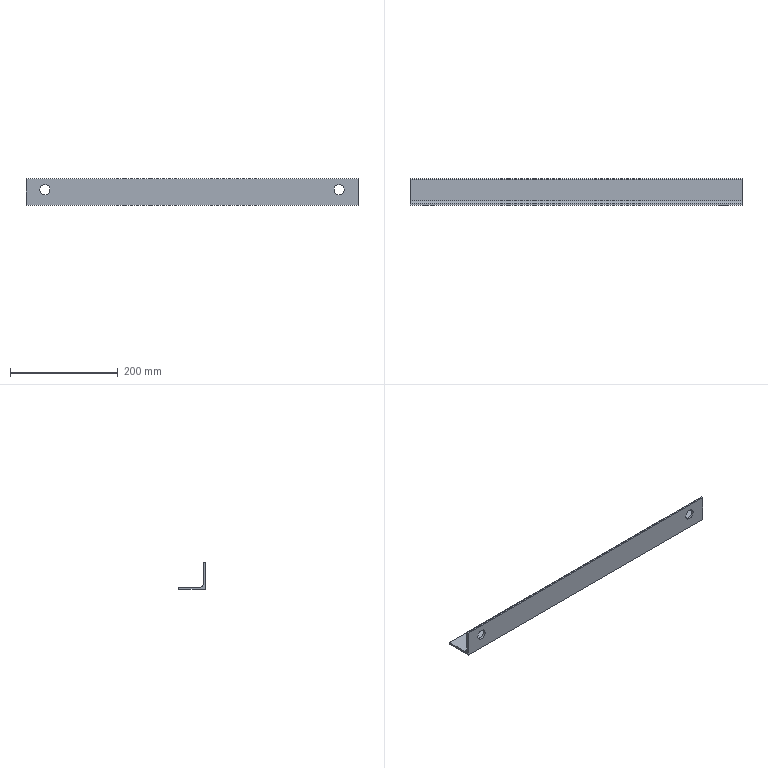Part | STEP file | Electrical cabinet angle steel 1_Default<As Machined> | 1 solid | 15 faces | box 617.5 x 50 x 50 mm | volume 238392 mm3 | plane 8 | cylinder 7 | commonest cylinder face diameters 19 x4 2.66 x2 11 x1
STEP:
#1=CARTESIAN_POINT('',(0.,0.,0.));
#2=DIRECTION('',(0.,0.,1.));
#3=DIRECTION('',(1.,0.,0.));
#4=AXIS2_PLACEMENT_3D('',#1,#2,#3);
#5=CARTESIAN_POINT('',(-273.75,0.,38.585));
#6=VERTEX_POINT('',#5);
#7=CARTESIAN_POINT('',(-273.75,4.,38.585));
#8=VERTEX_POINT('',#7);
#9=CARTESIAN_POINT('',(-273.75,-6.,38.585));
#10=DIRECTION('',(0.,1.,0.));
#11=VECTOR('',#10,1.);
#12=LINE('',#9,#11);
#13=CARTESIAN_POINT('',(-273.75,-6.,29.085));
#14=DIRECTION('',(0.,1.,0.));
#15=DIRECTION('',(0.,0.,1.));
#16=AXIS2_PLACEMENT_3D('',#13,#14,#15);
#17=CYLINDRICAL_SURFACE('',#16,9.5);
#18=CARTESIAN_POINT('',(6.283,0.));
#19=DIRECTION('',(0.,1.));
#20=VECTOR('',#19,1.);
#21=LINE('',#18,#20);
#22=(GEOMETRIC_REPRESENTATION_CONTEXT(2)PARAMETRIC_REPRESENTATION_CONTEXT()REPRESENTATION_CONTEXT('',''));
#23=DEFINITIONAL_REPRESENTATION('',(#21),#22);
#24=PCURVE('',#17,#23);
#25=CARTESIAN_POINT('',(-273.75,-6.,29.085));
#26=DIRECTION('',(0.,1.,0.));
#27=DIRECTION('',(0.,0.,1.));
#28=AXIS2_PLACEMENT_3D('',#25,#26,#27);
#29=CYLINDRICAL_SURFACE('',#28,9.5);
#30=CARTESIAN_POINT('',(0.,0.));
#31=DIRECTION('',(0.,1.));
#32=VECTOR('',#31,1.);
#33=LINE('',#30,#32);
#34=(GEOMETRIC_REPRESENTATION_CONTEXT(2)PARAMETRIC_REPRESENTATION_CONTEXT()REPRESENTATION_CONTEXT('',''));
#35=DEFINITIONAL_REPRESENTATION('',(#33),#34);
#36=PCURVE('',#29,#35);
#37=SURFACE_CURVE('',#12,(#24,#36),.PCURVE_S1.);
#38=EDGE_CURVE('',#6,#8,#37,.T.);
#39=ORIENTED_EDGE('',*,*,#38,.T.);
#40=CARTESIAN_POINT('',(-273.75,4.,19.585));
#41=VERTEX_POINT('',#40);
#42=CARTESIAN_POINT('',(-273.75,4.,29.085));
#43=DIRECTION('',(0.,1.,0.));
#44=DIRECTION('',(0.,0.,1.));
#45=AXIS2_PLACEMENT_3D('',#42,#43,#44);
#46=CIRCLE('',#45,9.5);
#47=CARTESIAN_POINT('',(0.,10.));
#48=DIRECTION('',(1.,0.));
#49=VECTOR('',#48,1.);
#50=LINE('',#47,#49);
#51=(GEOMETRIC_REPRESENTATION_CONTEXT(2)PARAMETRIC_REPRESENTATION_CONTEXT()REPRESENTATION_CONTEXT('',''));
#52=DEFINITIONAL_REPRESENTATION('',(#50),#51);
#53=PCURVE('',#17,#52);
#54=CARTESIAN_POINT('',(308.75,4.,48.67));
#55=DIRECTION('',(0.,-1.,0.));
#56=DIRECTION('',(1.,0.,0.));
#57=AXIS2_PLACEMENT_3D('',#54,#55,#56);
#58=PLANE('',#57);
#59=CARTESIAN_POINT('',(-582.5,-10.085));
#60=CARTESIAN_POINT('',(-566.046,-10.085));
#61=CARTESIAN_POINT('',(-574.273,-24.335));
#62=CARTESIAN_POINT('',(-582.5,-38.585));
#63=CARTESIAN_POINT('',(-590.727,-24.335));
#64=CARTESIAN_POINT('',(-598.954,-10.085));
#65=CARTESIAN_POINT('',(-582.5,-10.085));
#66=(BOUNDED_CURVE()B_SPLINE_CURVE(2,(#59,#60,#61,#62,#63,#64,#65),.UNSPECIFIED.,.T.,.F.)B_SPLINE_CURVE_WITH_KNOTS((1,2,2,2,2,1),(-2.094,0.,2.094,4.189,6.283,8.378),.UNSPECIFIED.)CURVE()GEOMETRIC_REPRESENTATION_ITEM()RATIONAL_B_SPLINE_CURVE((1.,0.5,1.,0.5,1.,0.5,1.))REPRESENTATION_ITEM(''));
#67=(GEOMETRIC_REPRESENTATION_CONTEXT(2)PARAMETRIC_REPRESENTATION_CONTEXT()REPRESENTATION_CONTEXT('',''));
#68=DEFINITIONAL_REPRESENTATION('',(#66),#67);
#69=PCURVE('',#58,#68);
#70=SURFACE_CURVE('',#46,(#53,#69),.PCURVE_S1.);
#71=EDGE_CURVE('',#41,#8,#70,.T.);
#72=ORIENTED_EDGE('',*,*,#71,.F.);
#73=CARTESIAN_POINT('',(-273.75,0.,19.585));
#74=VERTEX_POINT('',#73);
#75=CARTESIAN_POINT('',(-273.75,-6.,19.585));
#76=DIRECTION('',(0.,1.,0.));
#77=VECTOR('',#76,1.);
#78=LINE('',#75,#77);
#79=CARTESIAN_POINT('',(3.142,0.));
#80=DIRECTION('',(0.,1.));
#81=VECTOR('',#80,1.);
#82=LINE('',#79,#81);
#83=(GEOMETRIC_REPRESENTATION_CONTEXT(2)PARAMETRIC_REPRESENTATION_CONTEXT()REPRESENTATION_CONTEXT('',''));
#84=DEFINITIONAL_REPRESENTATION('',(#82),#83);
#85=PCURVE('',#17,#84);
#86=CARTESIAN_POINT('',(3.142,0.));
#87=DIRECTION('',(0.,1.));
#88=VECTOR('',#87,1.);
#89=LINE('',#86,#88);
#90=(GEOMETRIC_REPRESENTATION_CONTEXT(2)PARAMETRIC_REPRESENTATION_CONTEXT()REPRESENTATION_CONTEXT('',''));
#91=DEFINITIONAL_REPRESENTATION('',(#89),#90);
#92=PCURVE('',#29,#91);
#93=SURFACE_CURVE('',#78,(#85,#92),.PCURVE_S1.);
#94=EDGE_CURVE('',#74,#41,#93,.T.);
#95=ORIENTED_EDGE('',*,*,#94,.F.);
#96=CARTESIAN_POINT('',(-273.75,0.,29.085));
#97=DIRECTION('',(0.,1.,0.));
#98=DIRECTION('',(-1.,0.,0.));
#99=AXIS2_PLACEMENT_3D('',#96,#97,#98);
#100=CIRCLE('',#99,9.5);
#101=CARTESIAN_POINT('',(-1.571,6.));
#102=DIRECTION('',(1.,0.));
#103=VECTOR('',#102,1.);
#104=LINE('',#101,#103);
#105=(GEOMETRIC_REPRESENTATION_CONTEXT(2)PARAMETRIC_REPRESENTATION_CONTEXT()REPRESENTATION_CONTEXT('',''));
#106=DEFINITIONAL_REPRESENTATION('',(#104),#105);
#107=PCURVE('',#17,#106);
#108=CARTESIAN_POINT('',(308.75,0.,50.));
#109=DIRECTION('',(0.,1.,0.));
#110=DIRECTION('',(-1.,0.,0.));
#111=AXIS2_PLACEMENT_3D('',#108,#109,#110);
#112=PLANE('',#111);
#113=CARTESIAN_POINT('',(582.5,-20.915));
#114=DIRECTION('',(1.,0.));
#115=AXIS2_PLACEMENT_2D('',#113,#114);
#116=CIRCLE('',#115,9.5);
#117=(GEOMETRIC_REPRESENTATION_CONTEXT(2)PARAMETRIC_REPRESENTATION_CONTEXT()REPRESENTATION_CONTEXT('',''));
#118=DEFINITIONAL_REPRESENTATION('',(#116),#117);
#119=PCURVE('',#112,#118);
#120=SURFACE_CURVE('',#100,(#107,#119),.PCURVE_S1.);
#121=EDGE_CURVE('',#74,#6,#120,.T.);
#122=ORIENTED_EDGE('',*,*,#121,.T.);
#123=EDGE_LOOP('',(#39,#72,#95,#122));
#124=FACE_BOUND('',#123,.F.);
#125=ADVANCED_FACE('',(#124),#17,.F.);
#126=CARTESIAN_POINT('',(273.75,0.,38.585));
#127=VERTEX_POINT('',#126);
#128=CARTESIAN_POINT('',(273.75,4.,38.585));
#129=VERTEX_POINT('',#128);
#130=CARTESIAN_POINT('',(273.75,-6.,38.585));
#131=DIRECTION('',(0.,1.,0.));
#132=VECTOR('',#131,1.);
#133=LINE('',#130,#132);
#134=CARTESIAN_POINT('',(273.75,-6.,29.085));
#135=DIRECTION('',(0.,1.,0.));
#136=DIRECTION('',(0.,0.,1.));
#137=AXIS2_PLACEMENT_3D('',#134,#135,#136);
#138=CYLINDRICAL_SURFACE('',#137,9.5);
#139=CARTESIAN_POINT('',(6.283,0.));
#140=DIRECTION('',(0.,1.));
#141=VECTOR('',#140,1.);
#142=LINE('',#139,#141);
#143=(GEOMETRIC_REPRESENTATION_CONTEXT(2)PARAMETRIC_REPRESENTATION_CONTEXT()REPRESENTATION_CONTEXT('',''));
#144=DEFINITIONAL_REPRESENTATION('',(#142),#143);
#145=PCURVE('',#138,#144);
#146=CARTESIAN_POINT('',(273.75,-6.,29.085));
#147=DIRECTION('',(0.,1.,0.));
#148=DIRECTION('',(0.,0.,1.));
#149=AXIS2_PLACEMENT_3D('',#146,#147,#148);
#150=CYLINDRICAL_SURFACE('',#149,9.5);
#151=CARTESIAN_POINT('',(0.,0.));
#152=DIRECTION('',(0.,1.));
#153=VECTOR('',#152,1.);
#154=LINE('',#151,#153);
#155=(GEOMETRIC_REPRESENTATION_CONTEXT(2)PARAMETRIC_REPRESENTATION_CONTEXT()REPRESENTATION_CONTEXT('',''));
#156=DEFINITIONAL_REPRESENTATION('',(#154),#155);
#157=PCURVE('',#150,#156);
#158=SURFACE_CURVE('',#133,(#145,#157),.PCURVE_S1.);
#159=EDGE_CURVE('',#127,#129,#158,.T.);
#160=ORIENTED_EDGE('',*,*,#159,.T.);
#161=CARTESIAN_POINT('',(273.75,4.,19.585));
#162=VERTEX_POINT('',#161);
#163=CARTESIAN_POINT('',(273.75,4.,29.085));
#164=DIRECTION('',(0.,1.,0.));
#165=DIRECTION('',(0.,0.,-1.));
#166=AXIS2_PLACEMENT_3D('',#163,#164,#165);
#167=CIRCLE('',#166,9.5);
#168=CARTESIAN_POINT('',(3.142,10.));
#169=DIRECTION('',(1.,0.));
#170=VECTOR('',#169,1.);
#171=LINE('',#168,#170);
#172=(GEOMETRIC_REPRESENTATION_CONTEXT(2)PARAMETRIC_REPRESENTATION_CONTEXT()REPRESENTATION_CONTEXT('',''));
#173=DEFINITIONAL_REPRESENTATION('',(#171),#172);
#174=PCURVE('',#138,#173);
#175=CARTESIAN_POINT('',(-35.,-29.085));
#176=CARTESIAN_POINT('',(-51.454,-29.085));
#177=CARTESIAN_POINT('',(-43.227,-14.835));
#178=CARTESIAN_POINT('',(-35.,-0.585));
#179=CARTESIAN_POINT('',(-26.773,-14.835));
#180=CARTESIAN_POINT('',(-18.546,-29.085));
#181=CARTESIAN_POINT('',(-35.,-29.085));
#182=(BOUNDED_CURVE()B_SPLINE_CURVE(2,(#175,#176,#177,#178,#179,#180,#181),.UNSPECIFIED.,.T.,.F.)B_SPLINE_CURVE_WITH_KNOTS((1,2,2,2,2,1),(-2.094,0.,2.094,4.189,6.283,8.378),.UNSPECIFIED.)CURVE()GEOMETRIC_REPRESENTATION_ITEM()RATIONAL_B_SPLINE_CURVE((1.,0.5,1.,0.5,1.,0.5,1.))REPRESENTATION_ITEM(''));
#183=(GEOMETRIC_REPRESENTATION_CONTEXT(2)PARAMETRIC_REPRESENTATION_CONTEXT()REPRESENTATION_CONTEXT('',''));
#184=DEFINITIONAL_REPRESENTATION('',(#182),#183);
#185=PCURVE('',#58,#184);
#186=SURFACE_CURVE('',#167,(#174,#185),.PCURVE_S1.);
#187=EDGE_CURVE('',#162,#129,#186,.T.);
#188=ORIENTED_EDGE('',*,*,#187,.F.);
#189=CARTESIAN_POINT('',(273.75,0.,19.585));
#190=VERTEX_POINT('',#189);
#191=CARTESIAN_POINT('',(273.75,-6.,19.585));
#192=DIRECTION('',(0.,1.,0.));
#193=VECTOR('',#192,1.);
#194=LINE('',#191,#193);
#195=CARTESIAN_POINT('',(3.142,0.));
#196=DIRECTION('',(0.,1.));
#197=VECTOR('',#196,1.);
#198=LINE('',#195,#197);
#199=(GEOMETRIC_REPRESENTATION_CONTEXT(2)PARAMETRIC_REPRESENTATION_CONTEXT()REPRESENTATION_CONTEXT('',''));
#200=DEFINITIONAL_REPRESENTATION('',(#198),#199);
#201=PCURVE('',#138,#200);
#202=CARTESIAN_POINT('',(3.142,0.));
#203=DIRECTION('',(0.,1.));
#204=VECTOR('',#203,1.);
#205=LINE('',#202,#204);
#206=(GEOMETRIC_REPRESENTATION_CONTEXT(2)PARAMETRIC_REPRESENTATION_CONTEXT()REPRESENTATION_CONTEXT('',''));
#207=DEFINITIONAL_REPRESENTATION('',(#205),#206);
#208=PCURVE('',#150,#207);
#209=SURFACE_CURVE('',#194,(#201,#208),.PCURVE_S1.);
#210=EDGE_CURVE('',#190,#162,#209,.T.);
#211=ORIENTED_EDGE('',*,*,#210,.F.);
#212=CARTESIAN_POINT('',(273.75,0.,29.085));
#213=DIRECTION('',(0.,1.,0.));
#214=DIRECTION('',(-1.,0.,0.));
#215=AXIS2_PLACEMENT_3D('',#212,#213,#214);
#216=CIRCLE('',#215,9.5);
#217=CARTESIAN_POINT('',(-1.571,6.));
#218=DIRECTION('',(1.,0.));
#219=VECTOR('',#218,1.);
#220=LINE('',#217,#219);
#221=(GEOMETRIC_REPRESENTATION_CONTEXT(2)PARAMETRIC_REPRESENTATION_CONTEXT()REPRESENTATION_CONTEXT('',''));
#222=DEFINITIONAL_REPRESENTATION('',(#220),#221);
#223=PCURVE('',#138,#222);
#224=CARTESIAN_POINT('',(35.,-20.915));
#225=DIRECTION('',(1.,0.));
#226=AXIS2_PLACEMENT_2D('',#224,#225);
#227=CIRCLE('',#226,9.5);
#228=(GEOMETRIC_REPRESENTATION_CONTEXT(2)PARAMETRIC_REPRESENTATION_CONTEXT()REPRESENTATION_CONTEXT('',''));
#229=DEFINITIONAL_REPRESENTATION('',(#227),#228);
#230=PCURVE('',#112,#229);
#231=SURFACE_CURVE('',#216,(#223,#230),.PCURVE_S1.);
#232=EDGE_CURVE('',#190,#127,#231,.T.);
#233=ORIENTED_EDGE('',*,*,#232,.T.);
#234=EDGE_LOOP('',(#160,#188,#211,#233));
#235=FACE_BOUND('',#234,.F.);
#236=ADVANCED_FACE('',(#235),#138,.F.);
#237=CARTESIAN_POINT('',(-308.75,50.,2.67));
#238=VERTEX_POINT('',#237);
#239=CARTESIAN_POINT('',(-308.75,48.67,4.));
#240=VERTEX_POINT('',#239);
#241=CARTESIAN_POINT('',(-308.75,48.67,2.67));
#242=DIRECTION('',(1.,0.,0.));
#243=DIRECTION('',(0.,1.,0.));
#244=AXIS2_PLACEMENT_3D('',#241,#242,#243);
#245=CIRCLE('',#244,1.33);
#246=CARTESIAN_POINT('',(308.75,48.67,2.67));
#247=DIRECTION('',(-1.,0.,0.));
#248=DIRECTION('',(0.,-1.,0.));
#249=AXIS2_PLACEMENT_3D('',#246,#247,#248);
#250=CYLINDRICAL_SURFACE('',#249,1.33);
#251=CARTESIAN_POINT('',(3.142,617.5));
#252=DIRECTION('',(-1.,0.));
#253=VECTOR('',#252,1.);
#254=LINE('',#251,#253);
#255=(GEOMETRIC_REPRESENTATION_CONTEXT(2)PARAMETRIC_REPRESENTATION_CONTEXT()REPRESENTATION_CONTEXT('',''));
#256=DEFINITIONAL_REPRESENTATION('',(#254),#255);
#257=PCURVE('',#250,#256);
#258=CARTESIAN_POINT('',(-308.75,48.67,2.67));
#259=DIRECTION('',(1.,0.,0.));
#260=DIRECTION('',(0.,1.,0.));
#261=AXIS2_PLACEMENT_3D('',#258,#259,#260);
#262=PLANE('',#261);
#263=CARTESIAN_POINT('',(0.,0.));
#264=DIRECTION('',(1.,0.));
#265=AXIS2_PLACEMENT_2D('',#263,#264);
#266=CIRCLE('',#265,1.33);
#267=(GEOMETRIC_REPRESENTATION_CONTEXT(2)PARAMETRIC_REPRESENTATION_CONTEXT()REPRESENTATION_CONTEXT('',''));
#268=DEFINITIONAL_REPRESENTATION('',(#266),#267);
#269=PCURVE('',#262,#268);
#270=SURFACE_CURVE('',#245,(#257,#269),.PCURVE_S1.);
#271=EDGE_CURVE('',#238,#240,#270,.T.);
#272=ORIENTED_EDGE('',*,*,#271,.T.);
#273=CARTESIAN_POINT('',(308.75,48.67,4.));
#274=VERTEX_POINT('',#273);
#275=CARTESIAN_POINT('',(308.75,48.67,4.));
#276=DIRECTION('',(-1.,0.,0.));
#277=VECTOR('',#276,1.);
#278=LINE('',#275,#277);
#279=CARTESIAN_POINT('',(1.571,0.));
#280=DIRECTION('',(0.,1.));
#281=VECTOR('',#280,1.);
#282=LINE('',#279,#281);
#283=(GEOMETRIC_REPRESENTATION_CONTEXT(2)PARAMETRIC_REPRESENTATION_CONTEXT()REPRESENTATION_CONTEXT('',''));
#284=DEFINITIONAL_REPRESENTATION('',(#282),#283);
#285=PCURVE('',#250,#284);
#286=CARTESIAN_POINT('',(308.75,9.5,4.));
#287=DIRECTION('',(0.,0.,-1.));
#288=DIRECTION('',(-1.,0.,0.));
#289=AXIS2_PLACEMENT_3D('',#286,#287,#288);
#290=PLANE('',#289);
#291=CARTESIAN_POINT('',(0.,39.17));
#292=DIRECTION('',(1.,0.));
#293=VECTOR('',#292,1.);
#294=LINE('',#291,#293);
#295=(GEOMETRIC_REPRESENTATION_CONTEXT(2)PARAMETRIC_REPRESENTATION_CONTEXT()REPRESENTATION_CONTEXT('',''));
#296=DEFINITIONAL_REPRESENTATION('',(#294),#295);
#297=PCURVE('',#290,#296);
#298=SURFACE_CURVE('',#278,(#285,#297),.PCURVE_S1.);
#299=EDGE_CURVE('',#274,#240,#298,.T.);
#300=ORIENTED_EDGE('',*,*,#299,.F.);
#301=CARTESIAN_POINT('',(308.75,50.,2.67));
#302=VERTEX_POINT('',#301);
#303=CARTESIAN_POINT('',(308.75,48.67,2.67));
#304=DIRECTION('',(1.,0.,0.));
#305=DIRECTION('',(0.,1.,0.));
#306=AXIS2_PLACEMENT_3D('',#303,#304,#305);
#307=CIRCLE('',#306,1.33);
#308=CARTESIAN_POINT('',(3.142,0.));
#309=DIRECTION('',(-1.,0.));
#310=VECTOR('',#309,1.);
#311=LINE('',#308,#310);
#312=(GEOMETRIC_REPRESENTATION_CONTEXT(2)PARAMETRIC_REPRESENTATION_CONTEXT()REPRESENTATION_CONTEXT('',''));
#313=DEFINITIONAL_REPRESENTATION('',(#311),#312);
#314=PCURVE('',#250,#313);
#315=CARTESIAN_POINT('',(308.75,48.67,2.67));
#316=DIRECTION('',(1.,0.,0.));
#317=DIRECTION('',(0.,1.,0.));
#318=AXIS2_PLACEMENT_3D('',#315,#316,#317);
#319=PLANE('',#318);
#320=CARTESIAN_POINT('',(0.,0.));
#321=DIRECTION('',(1.,0.));
#322=AXIS2_PLACEMENT_2D('',#320,#321);
#323=CIRCLE('',#322,1.33);
#324=(GEOMETRIC_REPRESENTATION_CONTEXT(2)PARAMETRIC_REPRESENTATION_CONTEXT()REPRESENTATION_CONTEXT('',''));
#325=DEFINITIONAL_REPRESENTATION('',(#323),#324);
#326=PCURVE('',#319,#325);
#327=SURFACE_CURVE('',#307,(#314,#326),.PCURVE_S1.);
#328=EDGE_CURVE('',#302,#274,#327,.T.);
#329=ORIENTED_EDGE('',*,*,#328,.F.);
#330=CARTESIAN_POINT('',(308.75,50.,2.67));
#331=DIRECTION('',(-1.,0.,0.));
#332=VECTOR('',#331,1.);
#333=LINE('',#330,#332);
#334=CARTESIAN_POINT('',(3.142,0.));
#335=DIRECTION('',(0.,1.));
#336=VECTOR('',#335,1.);
#337=LINE('',#334,#336);
#338=(GEOMETRIC_REPRESENTATION_CONTEXT(2)PARAMETRIC_REPRESENTATION_CONTEXT()REPRESENTATION_CONTEXT('',''));
#339=DEFINITIONAL_REPRESENTATION('',(#337),#338);
#340=PCURVE('',#250,#339);
#341=CARTESIAN_POINT('',(308.75,50.,2.67));
#342=DIRECTION('',(0.,-1.,0.));
#343=DIRECTION('',(1.,0.,0.));
#344=AXIS2_PLACEMENT_3D('',#341,#342,#343);
#345=PLANE('',#344);
#346=CARTESIAN_POINT('',(0.,0.));
#347=DIRECTION('',(-1.,0.));
#348=VECTOR('',#347,1.);
#349=LINE('',#346,#348);
#350=(GEOMETRIC_REPRESENTATION_CONTEXT(2)PARAMETRIC_REPRESENTATION_CONTEXT()REPRESENTATION_CONTEXT('',''));
#351=DEFINITIONAL_REPRESENTATION('',(#349),#350);
#352=PCURVE('',#345,#351);
#353=SURFACE_CURVE('',#333,(#340,#352),.PCURVE_S1.);
#354=EDGE_CURVE('',#302,#238,#353,.T.);
#355=ORIENTED_EDGE('',*,*,#354,.T.);
#356=EDGE_LOOP('',(#272,#300,#329,#355));
#357=FACE_BOUND('',#356,.T.);
#358=ADVANCED_FACE('',(#357),#250,.T.);
#359=CARTESIAN_POINT('',(-308.75,9.5,4.));
#360=VERTEX_POINT('',#359);
#361=CARTESIAN_POINT('',(-308.75,9.5,4.));
#362=DIRECTION('',(0.,-1.,0.));
#363=VECTOR('',#362,1.);
#364=LINE('',#361,#363);
#365=CARTESIAN_POINT('',(617.5,0.));
#366=DIRECTION('',(0.,-1.));
#367=VECTOR('',#366,1.);
#368=LINE('',#365,#367);
#369=(GEOMETRIC_REPRESENTATION_CONTEXT(2)PARAMETRIC_REPRESENTATION_CONTEXT()REPRESENTATION_CONTEXT('',''));
#370=DEFINITIONAL_REPRESENTATION('',(#368),#369);
#371=PCURVE('',#290,#370);
#372=CARTESIAN_POINT('',(-39.17,1.33));
#373=DIRECTION('',(-1.,0.));
#374=VECTOR('',#373,1.);
#375=LINE('',#372,#374);
#376=(GEOMETRIC_REPRESENTATION_CONTEXT(2)PARAMETRIC_REPRESENTATION_CONTEXT()REPRESENTATION_CONTEXT('',''));
#377=DEFINITIONAL_REPRESENTATION('',(#375),#376);
#378=PCURVE('',#262,#377);
#379=SURFACE_CURVE('',#364,(#371,#378),.PCURVE_S1.);
#380=EDGE_CURVE('',#240,#360,#379,.T.);
#381=ORIENTED_EDGE('',*,*,#380,.T.);
#382=CARTESIAN_POINT('',(308.75,9.5,4.));
#383=VERTEX_POINT('',#382);
#384=CARTESIAN_POINT('',(308.75,9.5,4.));
#385=DIRECTION('',(-1.,0.,0.));
#386=VECTOR('',#385,1.);
#387=LINE('',#384,#386);
#388=CARTESIAN_POINT('',(0.,0.));
#389=DIRECTION('',(1.,0.));
#390=VECTOR('',#389,1.);
#391=LINE('',#388,#390);
#392=(GEOMETRIC_REPRESENTATION_CONTEXT(2)PARAMETRIC_REPRESENTATION_CONTEXT()REPRESENTATION_CONTEXT('',''));
#393=DEFINITIONAL_REPRESENTATION('',(#391),#392);
#394=PCURVE('',#290,#393);
#395=CARTESIAN_POINT('',(308.75,9.5,9.5));
#396=DIRECTION('',(-1.,0.,0.));
#397=DIRECTION('',(0.,-1.,0.));
#398=AXIS2_PLACEMENT_3D('',#395,#396,#397);
#399=CYLINDRICAL_SURFACE('',#398,5.5);
#400=CARTESIAN_POINT('',(4.712,0.));
#401=DIRECTION('',(0.,1.));
#402=VECTOR('',#401,1.);
#403=LINE('',#400,#402);
#404=(GEOMETRIC_REPRESENTATION_CONTEXT(2)PARAMETRIC_REPRESENTATION_CONTEXT()REPRESENTATION_CONTEXT('',''));
#405=DEFINITIONAL_REPRESENTATION('',(#403),#404);
#406=PCURVE('',#399,#405);
#407=SURFACE_CURVE('',#387,(#394,#406),.PCURVE_S1.);
#408=EDGE_CURVE('',#383,#360,#407,.T.);
#409=ORIENTED_EDGE('',*,*,#408,.F.);
#410=CARTESIAN_POINT('',(308.75,9.5,4.));
#411=DIRECTION('',(0.,-1.,0.));
#412=VECTOR('',#411,1.);
#413=LINE('',#410,#412);
#414=CARTESIAN_POINT('',(0.,0.));
#415=DIRECTION('',(0.,-1.));
#416=VECTOR('',#415,1.);
#417=LINE('',#414,#416);
#418=(GEOMETRIC_REPRESENTATION_CONTEXT(2)PARAMETRIC_REPRESENTATION_CONTEXT()REPRESENTATION_CONTEXT('',''));
#419=DEFINITIONAL_REPRESENTATION('',(#417),#418);
#420=PCURVE('',#290,#419);
#421=CARTESIAN_POINT('',(-39.17,1.33));
#422=DIRECTION('',(-1.,0.));
#423=VECTOR('',#422,1.);
#424=LINE('',#421,#423);
#425=(GEOMETRIC_REPRESENTATION_CONTEXT(2)PARAMETRIC_REPRESENTATION_CONTEXT()REPRESENTATION_CONTEXT('',''));
#426=DEFINITIONAL_REPRESENTATION('',(#424),#425);
#427=PCURVE('',#319,#426);
#428=SURFACE_CURVE('',#413,(#420,#427),.PCURVE_S1.);
#429=EDGE_CURVE('',#274,#383,#428,.T.);
#430=ORIENTED_EDGE('',*,*,#429,.F.);
#431=ORIENTED_EDGE('',*,*,#299,.T.);
#432=EDGE_LOOP('',(#381,#409,#430,#431));
#433=FACE_BOUND('',#432,.T.);
#434=ADVANCED_FACE('',(#433),#290,.F.);
#435=ORIENTED_EDGE('',*,*,#408,.F.);
#436=CARTESIAN_POINT('',(308.75,4.,9.5));
#437=VERTEX_POINT('',#436);
#438=CARTESIAN_POINT('',(308.75,9.5,9.5));
#439=DIRECTION('',(-1.,0.,0.));
#440=DIRECTION('',(0.,1.,0.));
#441=AXIS2_PLACEMENT_3D('',#438,#439,#440);
#442=CIRCLE('',#441,5.5);
#443=CARTESIAN_POINT('',(3.142,0.));
#444=DIRECTION('',(1.,0.));
#445=VECTOR('',#444,1.);
#446=LINE('',#443,#445);
#447=(GEOMETRIC_REPRESENTATION_CONTEXT(2)PARAMETRIC_REPRESENTATION_CONTEXT()REPRESENTATION_CONTEXT('',''));
#448=DEFINITIONAL_REPRESENTATION('',(#446),#447);
#449=PCURVE('',#399,#448);
#450=CARTESIAN_POINT('',(-33.67,6.83));
#451=CARTESIAN_POINT('',(-33.67,-2.696));
#452=CARTESIAN_POINT('',(-41.92,2.067));
#453=CARTESIAN_POINT('',(-50.17,6.83));
#454=CARTESIAN_POINT('',(-41.92,11.593));
#455=CARTESIAN_POINT('',(-33.67,16.356));
#456=CARTESIAN_POINT('',(-33.67,6.83));
#457=(BOUNDED_CURVE()B_SPLINE_CURVE(2,(#450,#451,#452,#453,#454,#455,#456),.UNSPECIFIED.,.T.,.F.)B_SPLINE_CURVE_WITH_KNOTS((1,2,2,2,2,1),(-2.094,0.,2.094,4.189,6.283,8.378),.UNSPECIFIED.)CURVE()GEOMETRIC_REPRESENTATION_ITEM()RATIONAL_B_SPLINE_CURVE((1.,0.5,1.,0.5,1.,0.5,1.))REPRESENTATION_ITEM(''));
#458=(GEOMETRIC_REPRESENTATION_CONTEXT(2)PARAMETRIC_REPRESENTATION_CONTEXT()REPRESENTATION_CONTEXT('',''));
#459=DEFINITIONAL_REPRESENTATION('',(#457),#458);
#460=PCURVE('',#319,#459);
#461=SURFACE_CURVE('',#442,(#449,#460),.PCURVE_S1.);
#462=EDGE_CURVE('',#383,#437,#461,.T.);
#463=ORIENTED_EDGE('',*,*,#462,.T.);
#464=CARTESIAN_POINT('',(-308.75,4.,9.5));
#465=VERTEX_POINT('',#464);
#466=CARTESIAN_POINT('',(308.75,4.,9.5));
#467=DIRECTION('',(-1.,0.,0.));
#468=VECTOR('',#467,1.);
#469=LINE('',#466,#468);
#470=CARTESIAN_POINT('',(6.283,0.));
#471=DIRECTION('',(0.,1.));
#472=VECTOR('',#471,1.);
#473=LINE('',#470,#472);
#474=(GEOMETRIC_REPRESENTATION_CONTEXT(2)PARAMETRIC_REPRESENTATION_CONTEXT()REPRESENTATION_CONTEXT('',''));
#475=DEFINITIONAL_REPRESENTATION('',(#473),#474);
#476=PCURVE('',#399,#475);
#477=CARTESIAN_POINT('',(0.,-39.17));
#478=DIRECTION('',(-1.,0.));
#479=VECTOR('',#478,1.);
#480=LINE('',#477,#479);
#481=(GEOMETRIC_REPRESENTATION_CONTEXT(2)PARAMETRIC_REPRESENTATION_CONTEXT()REPRESENTATION_CONTEXT('',''));
#482=DEFINITIONAL_REPRESENTATION('',(#480),#481);
#483=PCURVE('',#58,#482);
#484=SURFACE_CURVE('',#469,(#476,#483),.PCURVE_S1.);
#485=EDGE_CURVE('',#437,#465,#484,.T.);
#486=ORIENTED_EDGE('',*,*,#485,.T.);
#487=CARTESIAN_POINT('',(-308.75,9.5,9.5));
#488=DIRECTION('',(-1.,0.,0.));
#489=DIRECTION('',(0.,1.,0.));
#490=AXIS2_PLACEMENT_3D('',#487,#488,#489);
#491=CIRCLE('',#490,5.5);
#492=CARTESIAN_POINT('',(3.142,617.5));
#493=DIRECTION('',(1.,0.));
#494=VECTOR('',#493,1.);
#495=LINE('',#492,#494);
#496=(GEOMETRIC_REPRESENTATION_CONTEXT(2)PARAMETRIC_REPRESENTATION_CONTEXT()REPRESENTATION_CONTEXT('',''));
#497=DEFINITIONAL_REPRESENTATION('',(#495),#496);
#498=PCURVE('',#399,#497);
#499=CARTESIAN_POINT('',(-33.67,6.83));
#500=CARTESIAN_POINT('',(-33.67,-2.696));
#501=CARTESIAN_POINT('',(-41.92,2.067));
#502=CARTESIAN_POINT('',(-50.17,6.83));
#503=CARTESIAN_POINT('',(-41.92,11.593));
#504=CARTESIAN_POINT('',(-33.67,16.356));
#505=CARTESIAN_POINT('',(-33.67,6.83));
#506=(BOUNDED_CURVE()B_SPLINE_CURVE(2,(#499,#500,#501,#502,#503,#504,#505),.UNSPECIFIED.,.T.,.F.)B_SPLINE_CURVE_WITH_KNOTS((1,2,2,2,2,1),(-2.094,0.,2.094,4.189,6.283,8.378),.UNSPECIFIED.)CURVE()GEOMETRIC_REPRESENTATION_ITEM()RATIONAL_B_SPLINE_CURVE((1.,0.5,1.,0.5,1.,0.5,1.))REPRESENTATION_ITEM(''));
#507=(GEOMETRIC_REPRESENTATION_CONTEXT(2)PARAMETRIC_REPRESENTATION_CONTEXT()REPRESENTATION_CONTEXT('',''));
#508=DEFINITIONAL_REPRESENTATION('',(#506),#507);
#509=PCURVE('',#262,#508);
#510=SURFACE_CURVE('',#491,(#498,#509),.PCURVE_S1.);
#511=EDGE_CURVE('',#360,#465,#510,.T.);
#512=ORIENTED_EDGE('',*,*,#511,.F.);
#513=EDGE_LOOP('',(#435,#463,#486,#512));
#514=FACE_BOUND('',#513,.F.);
#515=ADVANCED_FACE('',(#514),#399,.F.);
#516=CARTESIAN_POINT('',(-273.75,4.,29.085));
#517=DIRECTION('',(0.,1.,0.));
#518=DIRECTION('',(0.,0.,1.));
#519=AXIS2_PLACEMENT_3D('',#516,#517,#518);
#520=CIRCLE('',#519,9.5);
#521=CARTESIAN_POINT('',(-582.5,-10.085));
#522=CARTESIAN_POINT('',(-566.046,-10.085));
#523=CARTESIAN_POINT('',(-574.273,-24.335));
#524=CARTESIAN_POINT('',(-582.5,-38.585));
#525=CARTESIAN_POINT('',(-590.727,-24.335));
#526=CARTESIAN_POINT('',(-598.954,-10.085));
#527=CARTESIAN_POINT('',(-582.5,-10.085));
#528=(BOUNDED_CURVE()B_SPLINE_CURVE(2,(#521,#522,#523,#524,#525,#526,#527),.UNSPECIFIED.,.T.,.F.)B_SPLINE_CURVE_WITH_KNOTS((1,2,2,2,2,1),(-2.094,0.,2.094,4.189,6.283,8.378),.UNSPECIFIED.)CURVE()GEOMETRIC_REPRESENTATION_ITEM()RATIONAL_B_SPLINE_CURVE((1.,0.5,1.,0.5,1.,0.5,1.))REPRESENTATION_ITEM(''));
#529=(GEOMETRIC_REPRESENTATION_CONTEXT(2)PARAMETRIC_REPRESENTATION_CONTEXT()REPRESENTATION_CONTEXT('',''));
#530=DEFINITIONAL_REPRESENTATION('',(#528),#529);
#531=PCURVE('',#58,#530);
#532=CARTESIAN_POINT('',(0.,10.));
#533=DIRECTION('',(1.,0.));
#534=VECTOR('',#533,1.);
#535=LINE('',#532,#534);
#536=(GEOMETRIC_REPRESENTATION_CONTEXT(2)PARAMETRIC_REPRESENTATION_CONTEXT()REPRESENTATION_CONTEXT('',''));
#537=DEFINITIONAL_REPRESENTATION('',(#535),#536);
#538=PCURVE('',#29,#537);
#539=SURFACE_CURVE('',#520,(#531,#538),.PCURVE_S1.);
#540=EDGE_CURVE('',#8,#41,#539,.T.);
#541=ORIENTED_EDGE('',*,*,#540,.F.);
#542=ORIENTED_EDGE('',*,*,#71,.F.);
#543=EDGE_LOOP('',(#541,#542));
#544=FACE_BOUND('',#543,.T.);
#545=CARTESIAN_POINT('',(273.75,4.,29.085));
#546=DIRECTION('',(0.,1.,0.));
#547=DIRECTION('',(0.,0.,-1.));
#548=AXIS2_PLACEMENT_3D('',#545,#546,#547);
#549=CIRCLE('',#548,9.5);
#550=CARTESIAN_POINT('',(-35.,-29.085));
#551=CARTESIAN_POINT('',(-51.454,-29.085));
#552=CARTESIAN_POINT('',(-43.227,-14.835));
#553=CARTESIAN_POINT('',(-35.,-0.585));
#554=CARTESIAN_POINT('',(-26.773,-14.835));
#555=CARTESIAN_POINT('',(-18.546,-29.085));
#556=CARTESIAN_POINT('',(-35.,-29.085));
#557=(BOUNDED_CURVE()B_SPLINE_CURVE(2,(#550,#551,#552,#553,#554,#555,#556),.UNSPECIFIED.,.T.,.F.)B_SPLINE_CURVE_WITH_KNOTS((1,2,2,2,2,1),(-2.094,0.,2.094,4.189,6.283,8.378),.UNSPECIFIED.)CURVE()GEOMETRIC_REPRESENTATION_ITEM()RATIONAL_B_SPLINE_CURVE((1.,0.5,1.,0.5,1.,0.5,1.))REPRESENTATION_ITEM(''));
#558=(GEOMETRIC_REPRESENTATION_CONTEXT(2)PARAMETRIC_REPRESENTATION_CONTEXT()REPRESENTATION_CONTEXT('',''));
#559=DEFINITIONAL_REPRESENTATION('',(#557),#558);
#560=PCURVE('',#58,#559);
#561=CARTESIAN_POINT('',(-3.142,10.));
#562=DIRECTION('',(1.,0.));
#563=VECTOR('',#562,1.);
#564=LINE('',#561,#563);
#565=(GEOMETRIC_REPRESENTATION_CONTEXT(2)PARAMETRIC_REPRESENTATION_CONTEXT()REPRESENTATION_CONTEXT('',''));
#566=DEFINITIONAL_REPRESENTATION('',(#564),#565);
#567=PCURVE('',#150,#566);
#568=SURFACE_CURVE('',#549,(#560,#567),.PCURVE_S1.);
#569=EDGE_CURVE('',#129,#162,#568,.T.);
#570=ORIENTED_EDGE('',*,*,#569,.F.);
#571=ORIENTED_EDGE('',*,*,#187,.F.);
#572=EDGE_LOOP('',(#570,#571));
#573=FACE_BOUND('',#572,.T.);
#574=CARTESIAN_POINT('',(-308.75,4.,48.67));
#575=VERTEX_POINT('',#574);
#576=CARTESIAN_POINT('',(-308.75,4.,48.67));
#577=DIRECTION('',(0.,0.,1.));
#578=VECTOR('',#577,1.);
#579=LINE('',#576,#578);
#580=CARTESIAN_POINT('',(-617.5,0.));
#581=DIRECTION('',(0.,1.));
#582=VECTOR('',#581,1.);
#583=LINE('',#580,#582);
#584=(GEOMETRIC_REPRESENTATION_CONTEXT(2)PARAMETRIC_REPRESENTATION_CONTEXT()REPRESENTATION_CONTEXT('',''));
#585=DEFINITIONAL_REPRESENTATION('',(#583),#584);
#586=PCURVE('',#58,#585);
#587=CARTESIAN_POINT('',(-44.67,46.));
#588=DIRECTION('',(0.,1.));
#589=VECTOR('',#588,1.);
#590=LINE('',#587,#589);
#591=(GEOMETRIC_REPRESENTATION_CONTEXT(2)PARAMETRIC_REPRESENTATION_CONTEXT()REPRESENTATION_CONTEXT('',''));
#592=DEFINITIONAL_REPRESENTATION('',(#590),#591);
#593=PCURVE('',#262,#592);
#594=SURFACE_CURVE('',#579,(#586,#593),.PCURVE_S1.);
#595=EDGE_CURVE('',#465,#575,#594,.T.);
#596=ORIENTED_EDGE('',*,*,#595,.T.);
#597=CARTESIAN_POINT('',(308.75,4.,48.67));
#598=VERTEX_POINT('',#597);
#599=CARTESIAN_POINT('',(308.75,4.,48.67));
#600=DIRECTION('',(-1.,0.,0.));
#601=VECTOR('',#600,1.);
#602=LINE('',#599,#601);
#603=CARTESIAN_POINT('',(0.,0.));
#604=DIRECTION('',(-1.,0.));
#605=VECTOR('',#604,1.);
#606=LINE('',#603,#605);
#607=(GEOMETRIC_REPRESENTATION_CONTEXT(2)PARAMETRIC_REPRESENTATION_CONTEXT()REPRESENTATION_CONTEXT('',''));
#608=DEFINITIONAL_REPRESENTATION('',(#606),#607);
#609=PCURVE('',#58,#608);
#610=CARTESIAN_POINT('',(308.75,2.67,48.67));
#611=DIRECTION('',(-1.,0.,0.));
#612=DIRECTION('',(0.,-1.,0.));
#613=AXIS2_PLACEMENT_3D('',#610,#611,#612);
#614=CYLINDRICAL_SURFACE('',#613,1.33);
#615=CARTESIAN_POINT('',(3.142,0.));
#616=DIRECTION('',(0.,1.));
#617=VECTOR('',#616,1.);
#618=LINE('',#615,#617);
#619=(GEOMETRIC_REPRESENTATION_CONTEXT(2)PARAMETRIC_REPRESENTATION_CONTEXT()REPRESENTATION_CONTEXT('',''));
#620=DEFINITIONAL_REPRESENTATION('',(#618),#619);
#621=PCURVE('',#614,#620);
#622=SURFACE_CURVE('',#602,(#609,#621),.PCURVE_S1.);
#623=EDGE_CURVE('',#598,#575,#622,.T.);
#624=ORIENTED_EDGE('',*,*,#623,.F.);
#625=CARTESIAN_POINT('',(308.75,4.,48.67));
#626=DIRECTION('',(0.,0.,1.));
#627=VECTOR('',#626,1.);
#628=LINE('',#625,#627);
#629=CARTESIAN_POINT('',(0.,0.));
#630=DIRECTION('',(0.,1.));
#631=VECTOR('',#630,1.);
#632=LINE('',#629,#631);
#633=(GEOMETRIC_REPRESENTATION_CONTEXT(2)PARAMETRIC_REPRESENTATION_CONTEXT()REPRESENTATION_CONTEXT('',''));
#634=DEFINITIONAL_REPRESENTATION('',(#632),#633);
#635=PCURVE('',#58,#634);
#636=CARTESIAN_POINT('',(-44.67,46.));
#637=DIRECTION('',(0.,1.));
#638=VECTOR('',#637,1.);
#639=LINE('',#636,#638);
#640=(GEOMETRIC_REPRESENTATION_CONTEXT(2)PARAMETRIC_REPRESENTATION_CONTEXT()REPRESENTATION_CONTEXT('',''));
#641=DEFINITIONAL_REPRESENTATION('',(#639),#640);
#642=PCURVE('',#319,#641);
#643=SURFACE_CURVE('',#628,(#635,#642),.PCURVE_S1.);
#644=EDGE_CURVE('',#437,#598,#643,.T.);
#645=ORIENTED_EDGE('',*,*,#644,.F.);
#646=ORIENTED_EDGE('',*,*,#485,.T.);
#647=EDGE_LOOP('',(#596,#624,#645,#646));
#648=FACE_BOUND('',#647,.T.);
#649=ADVANCED_FACE('',(#544,#573,#648),#58,.F.);
#650=CARTESIAN_POINT('',(-308.75,2.67,50.));
#651=VERTEX_POINT('',#650);
#652=CARTESIAN_POINT('',(-308.75,2.67,48.67));
#653=DIRECTION('',(1.,0.,0.));
#654=DIRECTION('',(0.,1.,0.));
#655=AXIS2_PLACEMENT_3D('',#652,#653,#654);
#656=CIRCLE('',#655,1.33);
#657=CARTESIAN_POINT('',(3.142,617.5));
#658=DIRECTION('',(-1.,0.));
#659=VECTOR('',#658,1.);
#660=LINE('',#657,#659);
#661=(GEOMETRIC_REPRESENTATION_CONTEXT(2)PARAMETRIC_REPRESENTATION_CONTEXT()REPRESENTATION_CONTEXT('',''));
#662=DEFINITIONAL_REPRESENTATION('',(#660),#661);
#663=PCURVE('',#614,#662);
#664=CARTESIAN_POINT('',(-46.,46.));
#665=DIRECTION('',(1.,0.));
#666=AXIS2_PLACEMENT_2D('',#664,#665);
#667=CIRCLE('',#666,1.33);
#668=(GEOMETRIC_REPRESENTATION_CONTEXT(2)PARAMETRIC_REPRESENTATION_CONTEXT()REPRESENTATION_CONTEXT('',''));
#669=DEFINITIONAL_REPRESENTATION('',(#667),#668);
#670=PCURVE('',#262,#669);
#671=SURFACE_CURVE('',#656,(#663,#670),.PCURVE_S1.);
#672=EDGE_CURVE('',#575,#651,#671,.T.);
#673=ORIENTED_EDGE('',*,*,#672,.T.);
#674=CARTESIAN_POINT('',(308.75,2.67,50.));
#675=VERTEX_POINT('',#674);
#676=CARTESIAN_POINT('',(308.75,2.67,50.));
#677=DIRECTION('',(-1.,0.,0.));
#678=VECTOR('',#677,1.);
#679=LINE('',#676,#678);
#680=CARTESIAN_POINT('',(1.571,0.));
#681=DIRECTION('',(0.,1.));
#682=VECTOR('',#681,1.);
#683=LINE('',#680,#682);
#684=(GEOMETRIC_REPRESENTATION_CONTEXT(2)PARAMETRIC_REPRESENTATION_CONTEXT()REPRESENTATION_CONTEXT('',''));
#685=DEFINITIONAL_REPRESENTATION('',(#683),#684);
#686=PCURVE('',#614,#685);
#687=CARTESIAN_POINT('',(308.75,0.,50.));
#688=DIRECTION('',(0.,0.,-1.));
#689=DIRECTION('',(0.,1.,0.));
#690=AXIS2_PLACEMENT_3D('',#687,#688,#689);
#691=PLANE('',#690);
#692=CARTESIAN_POINT('',(2.67,0.));
#693=DIRECTION('',(0.,-1.));
#694=VECTOR('',#693,1.);
#695=LINE('',#692,#694);
#696=(GEOMETRIC_REPRESENTATION_CONTEXT(2)PARAMETRIC_REPRESENTATION_CONTEXT()REPRESENTATION_CONTEXT('',''));
#697=DEFINITIONAL_REPRESENTATION('',(#695),#696);
#698=PCURVE('',#691,#697);
#699=SURFACE_CURVE('',#679,(#686,#698),.PCURVE_S1.);
#700=EDGE_CURVE('',#675,#651,#699,.T.);
#701=ORIENTED_EDGE('',*,*,#700,.F.);
#702=CARTESIAN_POINT('',(308.75,2.67,48.67));
#703=DIRECTION('',(1.,0.,0.));
#704=DIRECTION('',(0.,1.,0.));
#705=AXIS2_PLACEMENT_3D('',#702,#703,#704);
#706=CIRCLE('',#705,1.33);
#707=CARTESIAN_POINT('',(3.142,0.));
#708=DIRECTION('',(-1.,0.));
#709=VECTOR('',#708,1.);
#710=LINE('',#707,#709);
#711=(GEOMETRIC_REPRESENTATION_CONTEXT(2)PARAMETRIC_REPRESENTATION_CONTEXT()REPRESENTATION_CONTEXT('',''));
#712=DEFINITIONAL_REPRESENTATION('',(#710),#711);
#713=PCURVE('',#614,#712);
#714=CARTESIAN_POINT('',(-46.,46.));
#715=DIRECTION('',(1.,0.));
#716=AXIS2_PLACEMENT_2D('',#714,#715);
#717=CIRCLE('',#716,1.33);
#718=(GEOMETRIC_REPRESENTATION_CONTEXT(2)PARAMETRIC_REPRESENTATION_CONTEXT()REPRESENTATION_CONTEXT('',''));
#719=DEFINITIONAL_REPRESENTATION('',(#717),#718);
#720=PCURVE('',#319,#719);
#721=SURFACE_CURVE('',#706,(#713,#720),.PCURVE_S1.);
#722=EDGE_CURVE('',#598,#675,#721,.T.);
#723=ORIENTED_EDGE('',*,*,#722,.F.);
#724=ORIENTED_EDGE('',*,*,#623,.T.);
#725=EDGE_LOOP('',(#673,#701,#723,#724));
#726=FACE_BOUND('',#725,.T.);
#727=ADVANCED_FACE('',(#726),#614,.T.);
#728=CARTESIAN_POINT('',(-308.75,0.,50.));
#729=VERTEX_POINT('',#728);
#730=CARTESIAN_POINT('',(-308.75,0.,50.));
#731=DIRECTION('',(0.,-1.,0.));
#732=VECTOR('',#731,1.);
#733=LINE('',#730,#732);
#734=CARTESIAN_POINT('',(0.,-617.5));
#735=DIRECTION('',(-1.,0.));
#736=VECTOR('',#735,1.);
#737=LINE('',#734,#736);
#738=(GEOMETRIC_REPRESENTATION_CONTEXT(2)PARAMETRIC_REPRESENTATION_CONTEXT()REPRESENTATION_CONTEXT('',''));
#739=DEFINITIONAL_REPRESENTATION('',(#737),#738);
#740=PCURVE('',#691,#739);
#741=CARTESIAN_POINT('',(-48.67,47.33));
#742=DIRECTION('',(-1.,0.));
#743=VECTOR('',#742,1.);
#744=LINE('',#741,#743);
#745=(GEOMETRIC_REPRESENTATION_CONTEXT(2)PARAMETRIC_REPRESENTATION_CONTEXT()REPRESENTATION_CONTEXT('',''));
#746=DEFINITIONAL_REPRESENTATION('',(#744),#745);
#747=PCURVE('',#262,#746);
#748=SURFACE_CURVE('',#733,(#740,#747),.PCURVE_S1.);
#749=EDGE_CURVE('',#651,#729,#748,.T.);
#750=ORIENTED_EDGE('',*,*,#749,.T.);
#751=CARTESIAN_POINT('',(308.75,0.,50.));
#752=VERTEX_POINT('',#751);
#753=CARTESIAN_POINT('',(308.75,0.,50.));
#754=DIRECTION('',(-1.,0.,0.));
#755=VECTOR('',#754,1.);
#756=LINE('',#753,#755);
#757=CARTESIAN_POINT('',(0.,0.));
#758=DIRECTION('',(0.,-1.));
#759=VECTOR('',#758,1.);
#760=LINE('',#757,#759);
#761=(GEOMETRIC_REPRESENTATION_CONTEXT(2)PARAMETRIC_REPRESENTATION_CONTEXT()REPRESENTATION_CONTEXT('',''));
#762=DEFINITIONAL_REPRESENTATION('',(#760),#761);
#763=PCURVE('',#691,#762);
#764=CARTESIAN_POINT('',(0.,0.));
#765=DIRECTION('',(1.,0.));
#766=VECTOR('',#765,1.);
#767=LINE('',#764,#766);
#768=(GEOMETRIC_REPRESENTATION_CONTEXT(2)PARAMETRIC_REPRESENTATION_CONTEXT()REPRESENTATION_CONTEXT('',''));
#769=DEFINITIONAL_REPRESENTATION('',(#767),#768);
#770=PCURVE('',#112,#769);
#771=SURFACE_CURVE('',#756,(#763,#770),.PCURVE_S1.);
#772=EDGE_CURVE('',#752,#729,#771,.T.);
#773=ORIENTED_EDGE('',*,*,#772,.F.);
#774=CARTESIAN_POINT('',(308.75,0.,50.));
#775=DIRECTION('',(0.,-1.,0.));
#776=VECTOR('',#775,1.);
#777=LINE('',#774,#776);
#778=CARTESIAN_POINT('',(0.,0.));
#779=DIRECTION('',(-1.,0.));
#780=VECTOR('',#779,1.);
#781=LINE('',#778,#780);
#782=(GEOMETRIC_REPRESENTATION_CONTEXT(2)PARAMETRIC_REPRESENTATION_CONTEXT()REPRESENTATION_CONTEXT('',''));
#783=DEFINITIONAL_REPRESENTATION('',(#781),#782);
#784=PCURVE('',#691,#783);
#785=CARTESIAN_POINT('',(-48.67,47.33));
#786=DIRECTION('',(-1.,0.));
#787=VECTOR('',#786,1.);
#788=LINE('',#785,#787);
#789=(GEOMETRIC_REPRESENTATION_CONTEXT(2)PARAMETRIC_REPRESENTATION_CONTEXT()REPRESENTATION_CONTEXT('',''));
#790=DEFINITIONAL_REPRESENTATION('',(#788),#789);
#791=PCURVE('',#319,#790);
#792=SURFACE_CURVE('',#777,(#784,#791),.PCURVE_S1.);
#793=EDGE_CURVE('',#675,#752,#792,.T.);
#794=ORIENTED_EDGE('',*,*,#793,.F.);
#795=ORIENTED_EDGE('',*,*,#700,.T.);
#796=EDGE_LOOP('',(#750,#773,#794,#795));
#797=FACE_BOUND('',#796,.T.);
#798=ADVANCED_FACE('',(#797),#691,.F.);
#799=CARTESIAN_POINT('',(-273.75,0.,29.085));
#800=DIRECTION('',(0.,1.,0.));
#801=DIRECTION('',(-1.,0.,0.));
#802=AXIS2_PLACEMENT_3D('',#799,#800,#801);
#803=CIRCLE('',#802,9.5);
#804=CARTESIAN_POINT('',(582.5,-20.915));
#805=DIRECTION('',(1.,0.));
#806=AXIS2_PLACEMENT_2D('',#804,#805);
#807=CIRCLE('',#806,9.5);
#808=(GEOMETRIC_REPRESENTATION_CONTEXT(2)PARAMETRIC_REPRESENTATION_CONTEXT()REPRESENTATION_CONTEXT('',''));
#809=DEFINITIONAL_REPRESENTATION('',(#807),#808);
#810=PCURVE('',#112,#809);
#811=CARTESIAN_POINT('',(-1.571,6.));
#812=DIRECTION('',(1.,0.));
#813=VECTOR('',#812,1.);
#814=LINE('',#811,#813);
#815=(GEOMETRIC_REPRESENTATION_CONTEXT(2)PARAMETRIC_REPRESENTATION_CONTEXT()REPRESENTATION_CONTEXT('',''));
#816=DEFINITIONAL_REPRESENTATION('',(#814),#815);
#817=PCURVE('',#29,#816);
#818=SURFACE_CURVE('',#803,(#810,#817),.PCURVE_S1.);
#819=EDGE_CURVE('',#6,#74,#818,.T.);
#820=ORIENTED_EDGE('',*,*,#819,.T.);
#821=ORIENTED_EDGE('',*,*,#121,.T.);
#822=EDGE_LOOP('',(#820,#821));
#823=FACE_BOUND('',#822,.T.);
#824=CARTESIAN_POINT('',(273.75,0.,29.085));
#825=DIRECTION('',(0.,1.,0.));
#826=DIRECTION('',(-1.,0.,0.));
#827=AXIS2_PLACEMENT_3D('',#824,#825,#826);
#828=CIRCLE('',#827,9.5);
#829=CARTESIAN_POINT('',(35.,-20.915));
#830=DIRECTION('',(1.,0.));
#831=AXIS2_PLACEMENT_2D('',#829,#830);
#832=CIRCLE('',#831,9.5);
#833=(GEOMETRIC_REPRESENTATION_CONTEXT(2)PARAMETRIC_REPRESENTATION_CONTEXT()REPRESENTATION_CONTEXT('',''));
#834=DEFINITIONAL_REPRESENTATION('',(#832),#833);
#835=PCURVE('',#112,#834);
#836=CARTESIAN_POINT('',(-1.571,6.));
#837=DIRECTION('',(1.,0.));
#838=VECTOR('',#837,1.);
#839=LINE('',#836,#838);
#840=(GEOMETRIC_REPRESENTATION_CONTEXT(2)PARAMETRIC_REPRESENTATION_CONTEXT()REPRESENTATION_CONTEXT('',''));
#841=DEFINITIONAL_REPRESENTATION('',(#839),#840);
#842=PCURVE('',#150,#841);
#843=SURFACE_CURVE('',#828,(#835,#842),.PCURVE_S1.);
#844=EDGE_CURVE('',#127,#190,#843,.T.);
#845=ORIENTED_EDGE('',*,*,#844,.T.);
#846=ORIENTED_EDGE('',*,*,#232,.T.);
#847=EDGE_LOOP('',(#845,#846));
#848=FACE_BOUND('',#847,.T.);
#849=CARTESIAN_POINT('',(-308.75,0.,0.));
#850=VERTEX_POINT('',#849);
#851=CARTESIAN_POINT('',(-308.75,0.,50.));
#852=DIRECTION('',(0.,0.,-1.));
#853=VECTOR('',#852,1.);
#854=LINE('',#851,#853);
#855=CARTESIAN_POINT('',(617.5,0.));
#856=DIRECTION('',(0.,-1.));
#857=VECTOR('',#856,1.);
#858=LINE('',#855,#857);
#859=(GEOMETRIC_REPRESENTATION_CONTEXT(2)PARAMETRIC_REPRESENTATION_CONTEXT()REPRESENTATION_CONTEXT('',''));
#860=DEFINITIONAL_REPRESENTATION('',(#858),#859);
#861=PCURVE('',#112,#860);
#862=CARTESIAN_POINT('',(-48.67,47.33));
#863=DIRECTION('',(0.,-1.));
#864=VECTOR('',#863,1.);
#865=LINE('',#862,#864);
#866=(GEOMETRIC_REPRESENTATION_CONTEXT(2)PARAMETRIC_REPRESENTATION_CONTEXT()REPRESENTATION_CONTEXT('',''));
#867=DEFINITIONAL_REPRESENTATION('',(#865),#866);
#868=PCURVE('',#262,#867);
#869=SURFACE_CURVE('',#854,(#861,#868),.PCURVE_S1.);
#870=EDGE_CURVE('',#729,#850,#869,.T.);
#871=ORIENTED_EDGE('',*,*,#870,.T.);
#872=CARTESIAN_POINT('',(308.75,0.,0.));
#873=VERTEX_POINT('',#872);
#874=CARTESIAN_POINT('',(308.75,0.,0.));
#875=DIRECTION('',(-1.,0.,0.));
#876=VECTOR('',#875,1.);
#877=LINE('',#874,#876);
#878=CARTESIAN_POINT('',(0.,-50.));
#879=DIRECTION('',(1.,0.));
#880=VECTOR('',#879,1.);
#881=LINE('',#878,#880);
#882=(GEOMETRIC_REPRESENTATION_CONTEXT(2)PARAMETRIC_REPRESENTATION_CONTEXT()REPRESENTATION_CONTEXT('',''));
#883=DEFINITIONAL_REPRESENTATION('',(#881),#882);
#884=PCURVE('',#112,#883);
#885=CARTESIAN_POINT('',(308.75,0.,0.));
#886=DIRECTION('',(0.,0.,1.));
#887=DIRECTION('',(1.,0.,0.));
#888=AXIS2_PLACEMENT_3D('',#885,#886,#887);
#889=PLANE('',#888);
#890=CARTESIAN_POINT('',(0.,0.));
#891=DIRECTION('',(-1.,0.));
#892=VECTOR('',#891,1.);
#893=LINE('',#890,#892);
#894=(GEOMETRIC_REPRESENTATION_CONTEXT(2)PARAMETRIC_REPRESENTATION_CONTEXT()REPRESENTATION_CONTEXT('',''));
#895=DEFINITIONAL_REPRESENTATION('',(#893),#894);
#896=PCURVE('',#889,#895);
#897=SURFACE_CURVE('',#877,(#884,#896),.PCURVE_S1.);
#898=EDGE_CURVE('',#873,#850,#897,.T.);
#899=ORIENTED_EDGE('',*,*,#898,.F.);
#900=CARTESIAN_POINT('',(308.75,0.,50.));
#901=DIRECTION('',(0.,0.,-1.));
#902=VECTOR('',#901,1.);
#903=LINE('',#900,#902);
#904=CARTESIAN_POINT('',(0.,0.));
#905=DIRECTION('',(0.,-1.));
#906=VECTOR('',#905,1.);
#907=LINE('',#904,#906);
#908=(GEOMETRIC_REPRESENTATION_CONTEXT(2)PARAMETRIC_REPRESENTATION_CONTEXT()REPRESENTATION_CONTEXT('',''));
#909=DEFINITIONAL_REPRESENTATION('',(#907),#908);
#910=PCURVE('',#112,#909);
#911=CARTESIAN_POINT('',(-48.67,47.33));
#912=DIRECTION('',(0.,-1.));
#913=VECTOR('',#912,1.);
#914=LINE('',#911,#913);
#915=(GEOMETRIC_REPRESENTATION_CONTEXT(2)PARAMETRIC_REPRESENTATION_CONTEXT()REPRESENTATION_CONTEXT('',''));
#916=DEFINITIONAL_REPRESENTATION('',(#914),#915);
#917=PCURVE('',#319,#916);
#918=SURFACE_CURVE('',#903,(#910,#917),.PCURVE_S1.);
#919=EDGE_CURVE('',#752,#873,#918,.T.);
#920=ORIENTED_EDGE('',*,*,#919,.F.);
#921=ORIENTED_EDGE('',*,*,#772,.T.);
#922=EDGE_LOOP('',(#871,#899,#920,#921));
#923=FACE_BOUND('',#922,.T.);
#924=ADVANCED_FACE('',(#823,#848,#923),#112,.F.);
#925=CARTESIAN_POINT('',(-308.75,50.,0.));
#926=VERTEX_POINT('',#925);
#927=CARTESIAN_POINT('',(-308.75,0.,0.));
#928=DIRECTION('',(0.,1.,0.));
#929=VECTOR('',#928,1.);
#930=LINE('',#927,#929);
#931=CARTESIAN_POINT('',(-617.5,0.));
#932=DIRECTION('',(0.,1.));
#933=VECTOR('',#932,1.);
#934=LINE('',#931,#933);
#935=(GEOMETRIC_REPRESENTATION_CONTEXT(2)PARAMETRIC_REPRESENTATION_CONTEXT()REPRESENTATION_CONTEXT('',''));
#936=DEFINITIONAL_REPRESENTATION('',(#934),#935);
#937=PCURVE('',#889,#936);
#938=CARTESIAN_POINT('',(-48.67,-2.67));
#939=DIRECTION('',(1.,0.));
#940=VECTOR('',#939,1.);
#941=LINE('',#938,#940);
#942=(GEOMETRIC_REPRESENTATION_CONTEXT(2)PARAMETRIC_REPRESENTATION_CONTEXT()REPRESENTATION_CONTEXT('',''));
#943=DEFINITIONAL_REPRESENTATION('',(#941),#942);
#944=PCURVE('',#262,#943);
#945=SURFACE_CURVE('',#930,(#937,#944),.PCURVE_S1.);
#946=EDGE_CURVE('',#850,#926,#945,.T.);
#947=ORIENTED_EDGE('',*,*,#946,.T.);
#948=CARTESIAN_POINT('',(308.75,50.,0.));
#949=VERTEX_POINT('',#948);
#950=CARTESIAN_POINT('',(308.75,50.,0.));
#951=DIRECTION('',(-1.,0.,0.));
#952=VECTOR('',#951,1.);
#953=LINE('',#950,#952);
#954=CARTESIAN_POINT('',(0.,50.));
#955=DIRECTION('',(-1.,0.));
#956=VECTOR('',#955,1.);
#957=LINE('',#954,#956);
#958=(GEOMETRIC_REPRESENTATION_CONTEXT(2)PARAMETRIC_REPRESENTATION_CONTEXT()REPRESENTATION_CONTEXT('',''));
#959=DEFINITIONAL_REPRESENTATION('',(#957),#958);
#960=PCURVE('',#889,#959);
#961=CARTESIAN_POINT('',(0.,-2.67));
#962=DIRECTION('',(-1.,0.));
#963=VECTOR('',#962,1.);
#964=LINE('',#961,#963);
#965=(GEOMETRIC_REPRESENTATION_CONTEXT(2)PARAMETRIC_REPRESENTATION_CONTEXT()REPRESENTATION_CONTEXT('',''));
#966=DEFINITIONAL_REPRESENTATION('',(#964),#965);
#967=PCURVE('',#345,#966);
#968=SURFACE_CURVE('',#953,(#960,#967),.PCURVE_S1.);
#969=EDGE_CURVE('',#949,#926,#968,.T.);
#970=ORIENTED_EDGE('',*,*,#969,.F.);
#971=CARTESIAN_POINT('',(308.75,0.,0.));
#972=DIRECTION('',(0.,1.,0.));
#973=VECTOR('',#972,1.);
#974=LINE('',#971,#973);
#975=CARTESIAN_POINT('',(0.,0.));
#976=DIRECTION('',(0.,1.));
#977=VECTOR('',#976,1.);
#978=LINE('',#975,#977);
#979=(GEOMETRIC_REPRESENTATION_CONTEXT(2)PARAMETRIC_REPRESENTATION_CONTEXT()REPRESENTATION_CONTEXT('',''));
#980=DEFINITIONAL_REPRESENTATION('',(#978),#979);
#981=PCURVE('',#889,#980);
#982=CARTESIAN_POINT('',(-48.67,-2.67));
#983=DIRECTION('',(1.,0.));
#984=VECTOR('',#983,1.);
#985=LINE('',#982,#984);
#986=(GEOMETRIC_REPRESENTATION_CONTEXT(2)PARAMETRIC_REPRESENTATION_CONTEXT()REPRESENTATION_CONTEXT('',''));
#987=DEFINITIONAL_REPRESENTATION('',(#985),#986);
#988=PCURVE('',#319,#987);
#989=SURFACE_CURVE('',#974,(#981,#988),.PCURVE_S1.);
#990=EDGE_CURVE('',#873,#949,#989,.T.);
#991=ORIENTED_EDGE('',*,*,#990,.F.);
#992=ORIENTED_EDGE('',*,*,#898,.T.);
#993=EDGE_LOOP('',(#947,#970,#991,#992));
#994=FACE_BOUND('',#993,.T.);
#995=ADVANCED_FACE('',(#994),#889,.F.);
#996=CARTESIAN_POINT('',(-308.75,50.,2.67));
#997=DIRECTION('',(0.,0.,1.));
#998=VECTOR('',#997,1.);
#999=LINE('',#996,#998);
#1000=CARTESIAN_POINT('',(-617.5,0.));
#1001=DIRECTION('',(0.,1.));
#1002=VECTOR('',#1001,1.);
#1003=LINE('',#1000,#1002);
#1004=(GEOMETRIC_REPRESENTATION_CONTEXT(2)PARAMETRIC_REPRESENTATION_CONTEXT()REPRESENTATION_CONTEXT('',''));
#1005=DEFINITIONAL_REPRESENTATION('',(#1003),#1004);
#1006=PCURVE('',#345,#1005);
#1007=CARTESIAN_POINT('',(1.33,0.));
#1008=DIRECTION('',(0.,1.));
#1009=VECTOR('',#1008,1.);
#1010=LINE('',#1007,#1009);
#1011=(GEOMETRIC_REPRESENTATION_CONTEXT(2)PARAMETRIC_REPRESENTATION_CONTEXT()REPRESENTATION_CONTEXT('',''));
#1012=DEFINITIONAL_REPRESENTATION('',(#1010),#1011);
#1013=PCURVE('',#262,#1012);
#1014=SURFACE_CURVE('',#999,(#1006,#1013),.PCURVE_S1.);
#1015=EDGE_CURVE('',#926,#238,#1014,.T.);
#1016=ORIENTED_EDGE('',*,*,#1015,.T.);
#1017=ORIENTED_EDGE('',*,*,#354,.F.);
#1018=CARTESIAN_POINT('',(308.75,50.,2.67));
#1019=DIRECTION('',(0.,0.,1.));
#1020=VECTOR('',#1019,1.);
#1021=LINE('',#1018,#1020);
#1022=CARTESIAN_POINT('',(0.,0.));
#1023=DIRECTION('',(0.,1.));
#1024=VECTOR('',#1023,1.);
#1025=LINE('',#1022,#1024);
#1026=(GEOMETRIC_REPRESENTATION_CONTEXT(2)PARAMETRIC_REPRESENTATION_CONTEXT()REPRESENTATION_CONTEXT('',''));
#1027=DEFINITIONAL_REPRESENTATION('',(#1025),#1026);
#1028=PCURVE('',#345,#1027);
#1029=CARTESIAN_POINT('',(1.33,0.));
#1030=DIRECTION('',(0.,1.));
#1031=VECTOR('',#1030,1.);
#1032=LINE('',#1029,#1031);
#1033=(GEOMETRIC_REPRESENTATION_CONTEXT(2)PARAMETRIC_REPRESENTATION_CONTEXT()REPRESENTATION_CONTEXT('',''));
#1034=DEFINITIONAL_REPRESENTATION('',(#1032),#1033);
#1035=PCURVE('',#319,#1034);
#1036=SURFACE_CURVE('',#1021,(#1028,#1035),.PCURVE_S1.);
#1037=EDGE_CURVE('',#949,#302,#1036,.T.);
#1038=ORIENTED_EDGE('',*,*,#1037,.F.);
#1039=ORIENTED_EDGE('',*,*,#969,.T.);
#1040=EDGE_LOOP('',(#1016,#1017,#1038,#1039));
#1041=FACE_BOUND('',#1040,.T.);
#1042=ADVANCED_FACE('',(#1041),#345,.F.);
#1043=ORIENTED_EDGE('',*,*,#328,.T.);
#1044=ORIENTED_EDGE('',*,*,#429,.T.);
#1045=ORIENTED_EDGE('',*,*,#462,.T.);
#1046=ORIENTED_EDGE('',*,*,#644,.T.);
#1047=ORIENTED_EDGE('',*,*,#722,.T.);
#1048=ORIENTED_EDGE('',*,*,#793,.T.);
#1049=ORIENTED_EDGE('',*,*,#919,.T.);
#1050=ORIENTED_EDGE('',*,*,#990,.T.);
#1051=ORIENTED_EDGE('',*,*,#1037,.T.);
#1052=EDGE_LOOP('',(#1043,#1044,#1045,#1046,#1047,#1048,#1049,#1050,#1051));
#1053=FACE_BOUND('',#1052,.T.);
#1054=ADVANCED_FACE('',(#1053),#319,.T.);
#1055=ORIENTED_EDGE('',*,*,#271,.F.);
#1056=ORIENTED_EDGE('',*,*,#1015,.F.);
#1057=ORIENTED_EDGE('',*,*,#946,.F.);
#1058=ORIENTED_EDGE('',*,*,#870,.F.);
#1059=ORIENTED_EDGE('',*,*,#749,.F.);
#1060=ORIENTED_EDGE('',*,*,#672,.F.);
#1061=ORIENTED_EDGE('',*,*,#595,.F.);
#1062=ORIENTED_EDGE('',*,*,#511,.F.);
#1063=ORIENTED_EDGE('',*,*,#380,.F.);
#1064=EDGE_LOOP('',(#1055,#1056,#1057,#1058,#1059,#1060,#1061,#1062,#1063));
#1065=FACE_BOUND('',#1064,.T.);
#1066=ADVANCED_FACE('',(#1065),#262,.F.);
#1067=ORIENTED_EDGE('',*,*,#569,.F.);
#1068=ORIENTED_EDGE('',*,*,#159,.F.);
#1069=ORIENTED_EDGE('',*,*,#844,.T.);
#1070=ORIENTED_EDGE('',*,*,#210,.T.);
#1071=EDGE_LOOP('',(#1067,#1068,#1069,#1070));
#1072=FACE_BOUND('',#1071,.F.);
#1073=ADVANCED_FACE('',(#1072),#150,.F.);
#1074=ORIENTED_EDGE('',*,*,#540,.F.);
#1075=ORIENTED_EDGE('',*,*,#38,.F.);
#1076=ORIENTED_EDGE('',*,*,#819,.T.);
#1077=ORIENTED_EDGE('',*,*,#94,.T.);
#1078=EDGE_LOOP('',(#1074,#1075,#1076,#1077));
#1079=FACE_BOUND('',#1078,.F.);
#1080=ADVANCED_FACE('',(#1079),#29,.F.);
#1081=CLOSED_SHELL('',(#125,#236,#358,#434,#515,#649,#727,#798,#924,#995,#1042,#1054,#1066,#1073,#1080));
#1082=MANIFOLD_SOLID_BREP('',#1081);
#1083=(LENGTH_UNIT()NAMED_UNIT(*)SI_UNIT(.MILLI.,.METRE.));
#1084=UNCERTAINTY_MEASURE_WITH_UNIT(LENGTH_MEASURE(0.0000001),#1083,'','');
#1085=(NAMED_UNIT(*)PLANE_ANGLE_UNIT()SI_UNIT($,.RADIAN.));
#1086=(NAMED_UNIT(*)SI_UNIT($,.STERADIAN.)SOLID_ANGLE_UNIT());
#1087=(GEOMETRIC_REPRESENTATION_CONTEXT(3)GLOBAL_UNCERTAINTY_ASSIGNED_CONTEXT((#1084))GLOBAL_UNIT_ASSIGNED_CONTEXT((#1083,#1085,#1086))REPRESENTATION_CONTEXT('',''));
#1088=ADVANCED_BREP_SHAPE_REPRESENTATION('',(#4,#1082),#1087);